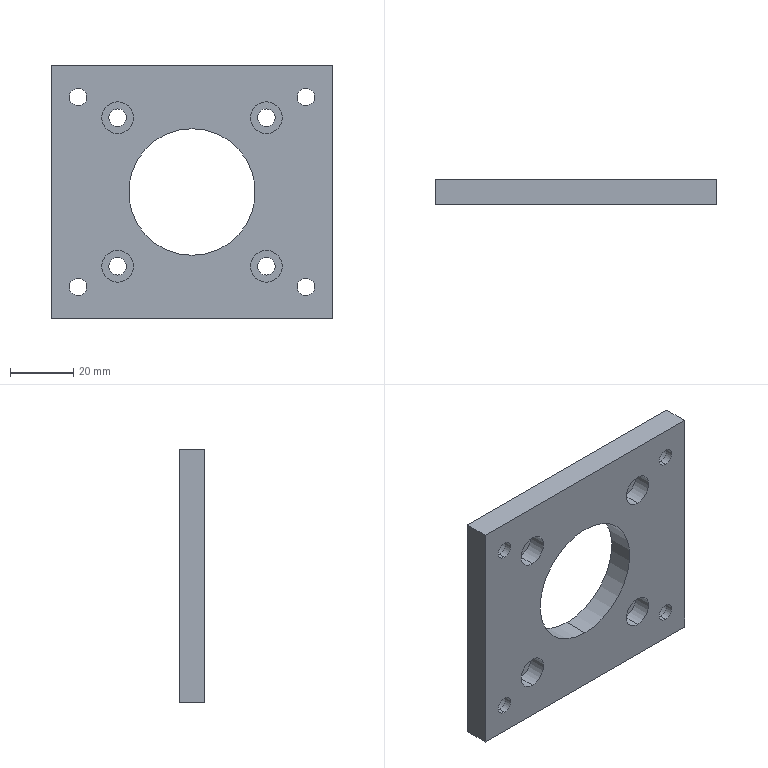Part | STEP file | PN_0008 motor plate | 1 solid | 48 faces | box 89 x 8 x 80 mm | volume 42888 mm3 | cylinder 34 | plane 14 | commonest cylinder face diameters 5.5 x16 10 x16 40 x2